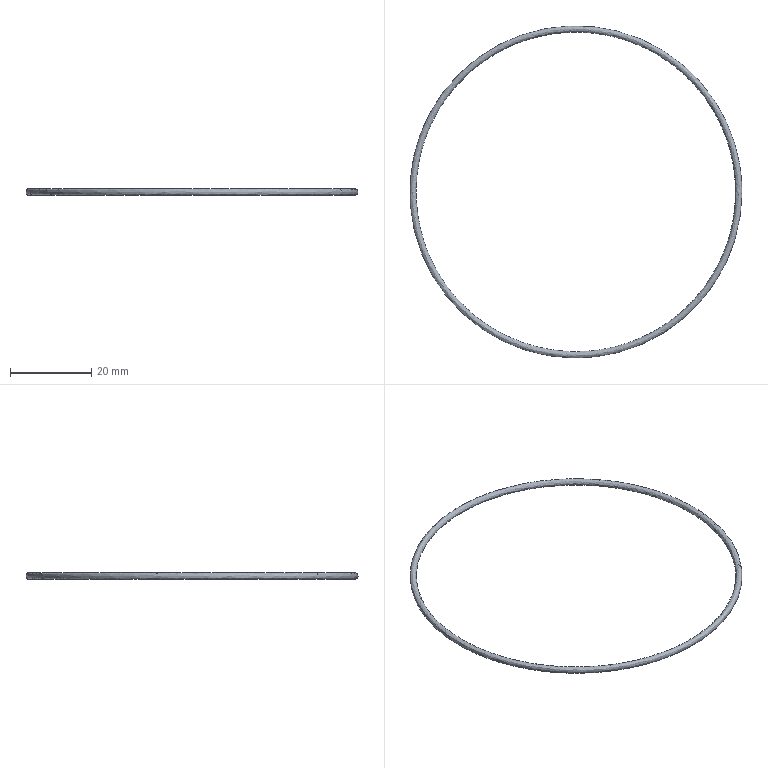Part | NX | features DATUM_CSYS 3, SKETCH 2, SKIN 1 | 1 solid | 1 faces | box 81.599 x 81.597 x 1.6 mm | volume 504.996 mm3 | spline 1